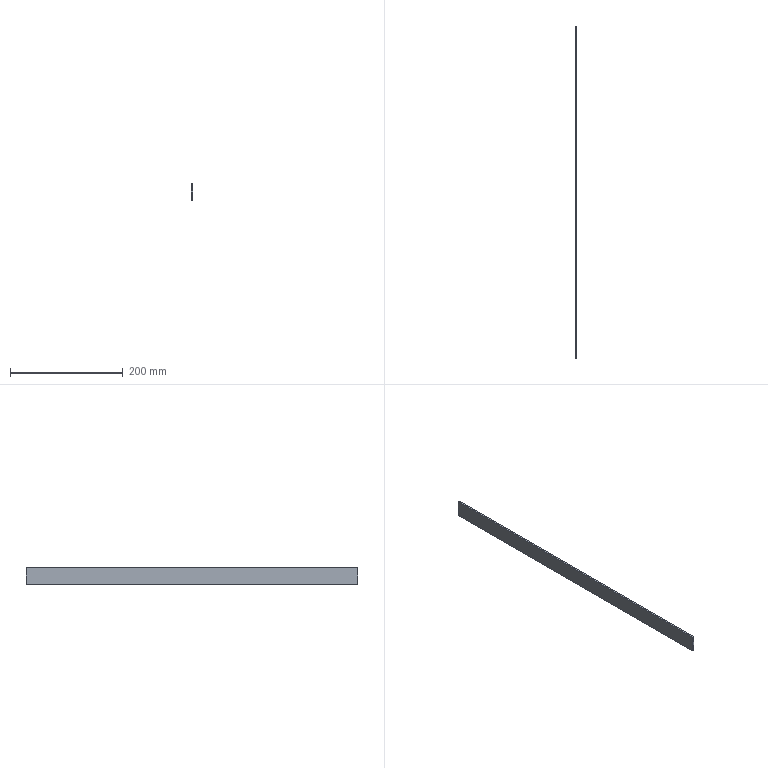Part | SolidWorks | 1 solid | 6 faces | box 3 x 590 x 30 mm | volume 53100 mm3 | plane 6
STEP:
#1=CARTESIAN_POINT('',(0.,295.,15.));
#2=VERTEX_POINT('',#1);
#3=CARTESIAN_POINT('',(0.,-295.,15.));
#4=VERTEX_POINT('',#3);
#5=CARTESIAN_POINT('',(0.,-295.,15.));
#6=DIRECTION('',(0.,-1.,0.));
#7=VECTOR('',#6,1000.);
#8=LINE('',#5,#7);
#9=EDGE_CURVE('',#2,#4,#8,.T.);
#10=ORIENTED_EDGE('',*,*,#9,.F.);
#11=CARTESIAN_POINT('',(-3.,295.,15.));
#12=VERTEX_POINT('',#11);
#13=CARTESIAN_POINT('',(-3.,295.,15.));
#14=DIRECTION('',(1.,0.,0.));
#15=VECTOR('',#14,1000.);
#16=LINE('',#13,#15);
#17=EDGE_CURVE('',#12,#2,#16,.T.);
#18=ORIENTED_EDGE('',*,*,#17,.F.);
#19=CARTESIAN_POINT('',(-3.,-295.,15.));
#20=VERTEX_POINT('',#19);
#21=CARTESIAN_POINT('',(-3.,-295.,15.));
#22=DIRECTION('',(0.,-1.,0.));
#23=VECTOR('',#22,1000.);
#24=LINE('',#21,#23);
#25=EDGE_CURVE('',#12,#20,#24,.T.);
#26=ORIENTED_EDGE('',*,*,#25,.T.);
#27=CARTESIAN_POINT('',(-3.,-295.,15.));
#28=DIRECTION('',(1.,0.,0.));
#29=VECTOR('',#28,1000.);
#30=LINE('',#27,#29);
#31=EDGE_CURVE('',#20,#4,#30,.T.);
#32=ORIENTED_EDGE('',*,*,#31,.T.);
#33=EDGE_LOOP('',(#10,#18,#26,#32));
#34=FACE_OUTER_BOUND('',#33,.T.);
#35=CARTESIAN_POINT('',(-3.,-295.,15.));
#36=DIRECTION('',(0.,0.,1.));
#37=DIRECTION('',(1.,0.,0.));
#38=AXIS2_PLACEMENT_3D('',#35,#36,#37);
#39=PLANE('',#38);
#40=ADVANCED_FACE('',(#34),#39,.T.);
#41=CARTESIAN_POINT('',(0.,295.,-15.));
#42=VERTEX_POINT('',#41);
#43=CARTESIAN_POINT('',(0.,295.,-15.));
#44=DIRECTION('',(0.,0.,1.));
#45=VECTOR('',#44,1000.);
#46=LINE('',#43,#45);
#47=EDGE_CURVE('',#42,#2,#46,.T.);
#48=ORIENTED_EDGE('',*,*,#47,.F.);
#49=CARTESIAN_POINT('',(-3.,295.,-15.));
#50=VERTEX_POINT('',#49);
#51=CARTESIAN_POINT('',(-3.,295.,-15.));
#52=DIRECTION('',(1.,0.,0.));
#53=VECTOR('',#52,1000.);
#54=LINE('',#51,#53);
#55=EDGE_CURVE('',#50,#42,#54,.T.);
#56=ORIENTED_EDGE('',*,*,#55,.F.);
#57=CARTESIAN_POINT('',(-3.,295.,-15.));
#58=DIRECTION('',(0.,0.,1.));
#59=VECTOR('',#58,1000.);
#60=LINE('',#57,#59);
#61=EDGE_CURVE('',#50,#12,#60,.T.);
#62=ORIENTED_EDGE('',*,*,#61,.T.);
#63=ORIENTED_EDGE('',*,*,#17,.T.);
#64=EDGE_LOOP('',(#48,#56,#62,#63));
#65=FACE_OUTER_BOUND('',#64,.T.);
#66=CARTESIAN_POINT('',(-3.,295.,-15.));
#67=DIRECTION('',(0.,1.,0.));
#68=DIRECTION('',(0.,0.,1.));
#69=AXIS2_PLACEMENT_3D('',#66,#67,#68);
#70=PLANE('',#69);
#71=ADVANCED_FACE('',(#65),#70,.T.);
#72=CARTESIAN_POINT('',(0.,-295.,-15.));
#73=VERTEX_POINT('',#72);
#74=CARTESIAN_POINT('',(0.,-295.,-15.));
#75=DIRECTION('',(0.,1.,0.));
#76=VECTOR('',#75,1000.);
#77=LINE('',#74,#76);
#78=EDGE_CURVE('',#73,#42,#77,.T.);
#79=ORIENTED_EDGE('',*,*,#78,.F.);
#80=CARTESIAN_POINT('',(-3.,-295.,-15.));
#81=VERTEX_POINT('',#80);
#82=CARTESIAN_POINT('',(-3.,-295.,-15.));
#83=DIRECTION('',(1.,0.,0.));
#84=VECTOR('',#83,1000.);
#85=LINE('',#82,#84);
#86=EDGE_CURVE('',#81,#73,#85,.T.);
#87=ORIENTED_EDGE('',*,*,#86,.F.);
#88=CARTESIAN_POINT('',(-3.,-295.,-15.));
#89=DIRECTION('',(0.,1.,0.));
#90=VECTOR('',#89,1000.);
#91=LINE('',#88,#90);
#92=EDGE_CURVE('',#81,#50,#91,.T.);
#93=ORIENTED_EDGE('',*,*,#92,.T.);
#94=ORIENTED_EDGE('',*,*,#55,.T.);
#95=EDGE_LOOP('',(#79,#87,#93,#94));
#96=FACE_OUTER_BOUND('',#95,.T.);
#97=CARTESIAN_POINT('',(-3.,-295.,-15.));
#98=DIRECTION('',(0.,0.,-1.));
#99=DIRECTION('',(-1.,0.,0.));
#100=AXIS2_PLACEMENT_3D('',#97,#98,#99);
#101=PLANE('',#100);
#102=ADVANCED_FACE('',(#96),#101,.T.);
#103=CARTESIAN_POINT('',(0.,-295.,-15.));
#104=DIRECTION('',(0.,0.,-1.));
#105=VECTOR('',#104,1000.);
#106=LINE('',#103,#105);
#107=EDGE_CURVE('',#4,#73,#106,.T.);
#108=ORIENTED_EDGE('',*,*,#107,.F.);
#109=ORIENTED_EDGE('',*,*,#31,.F.);
#110=CARTESIAN_POINT('',(-3.,-295.,-15.));
#111=DIRECTION('',(0.,0.,-1.));
#112=VECTOR('',#111,1000.);
#113=LINE('',#110,#112);
#114=EDGE_CURVE('',#20,#81,#113,.T.);
#115=ORIENTED_EDGE('',*,*,#114,.T.);
#116=ORIENTED_EDGE('',*,*,#86,.T.);
#117=EDGE_LOOP('',(#108,#109,#115,#116));
#118=FACE_OUTER_BOUND('',#117,.T.);
#119=CARTESIAN_POINT('',(-3.,-295.,-15.));
#120=DIRECTION('',(0.,-1.,0.));
#121=DIRECTION('',(0.,0.,-1.));
#122=AXIS2_PLACEMENT_3D('',#119,#120,#121);
#123=PLANE('',#122);
#124=ADVANCED_FACE('',(#118),#123,.T.);
#125=ORIENTED_EDGE('',*,*,#25,.F.);
#126=ORIENTED_EDGE('',*,*,#61,.F.);
#127=ORIENTED_EDGE('',*,*,#92,.F.);
#128=ORIENTED_EDGE('',*,*,#114,.F.);
#129=EDGE_LOOP('',(#125,#126,#127,#128));
#130=FACE_OUTER_BOUND('',#129,.T.);
#131=CARTESIAN_POINT('',(-3.,0.,0.));
#132=DIRECTION('',(1.,0.,0.));
#133=DIRECTION('',(0.,0.,-1.));
#134=AXIS2_PLACEMENT_3D('',#131,#132,#133);
#135=PLANE('',#134);
#136=ADVANCED_FACE('',(#130),#135,.F.);
#137=ORIENTED_EDGE('',*,*,#9,.T.);
#138=ORIENTED_EDGE('',*,*,#107,.T.);
#139=ORIENTED_EDGE('',*,*,#78,.T.);
#140=ORIENTED_EDGE('',*,*,#47,.T.);
#141=EDGE_LOOP('',(#137,#138,#139,#140));
#142=FACE_OUTER_BOUND('',#141,.T.);
#143=CARTESIAN_POINT('',(0.,0.,0.));
#144=DIRECTION('',(1.,0.,0.));
#145=DIRECTION('',(0.,0.,-1.));
#146=AXIS2_PLACEMENT_3D('',#143,#144,#145);
#147=PLANE('',#146);
#148=ADVANCED_FACE('',(#142),#147,.T.);
#149=CLOSED_SHELL('',(#40,#71,#102,#124,#136,#148));
#150=MANIFOLD_SOLID_BREP('',#149);
#151=CARTESIAN_POINT('',(0.,0.,0.));
#152=DIRECTION('',(0.,0.,1.));
#153=DIRECTION('',(1.,0.,0.));
#154=AXIS2_PLACEMENT_3D('',#151,#152,#153);
#155=(LENGTH_UNIT()NAMED_UNIT(*)SI_UNIT(.MILLI.,.METRE.));
#156=UNCERTAINTY_MEASURE_WITH_UNIT(LENGTH_MEASURE(0.00001),#155,'','');
#157=(NAMED_UNIT(*)PLANE_ANGLE_UNIT()SI_UNIT($,.RADIAN.));
#158=(NAMED_UNIT(*)SI_UNIT($,.STERADIAN.)SOLID_ANGLE_UNIT());
#159=(GEOMETRIC_REPRESENTATION_CONTEXT(3)GLOBAL_UNCERTAINTY_ASSIGNED_CONTEXT((#156))GLOBAL_UNIT_ASSIGNED_CONTEXT((#155,#157,#158))REPRESENTATION_CONTEXT('',''));
#160=ADVANCED_BREP_SHAPE_REPRESENTATION('',(#150,#154),#159);